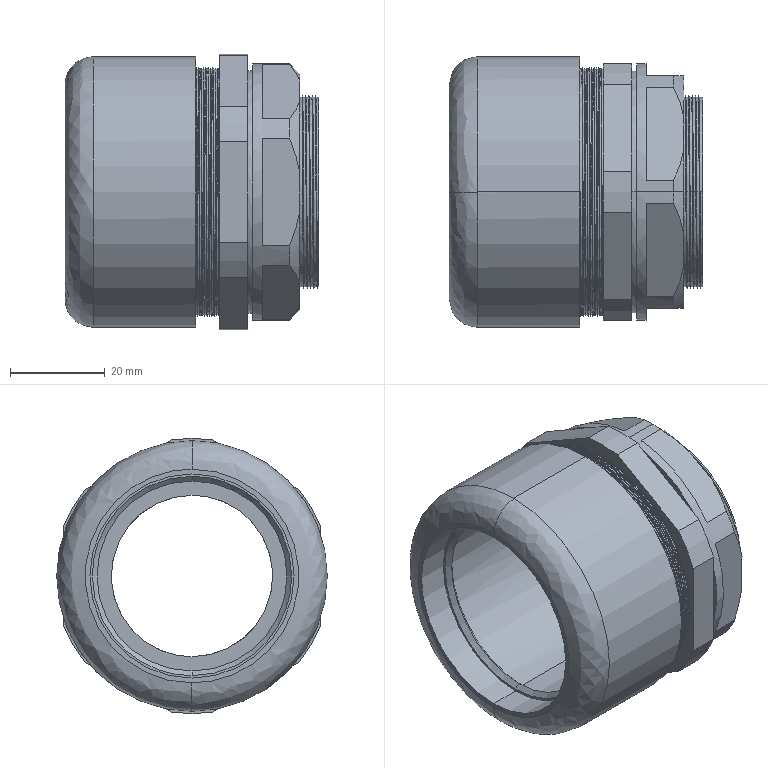Part | SolidWorks | features BaseBody 1 | 1 solid | 106 faces | box 53.5 x 57 x 57.999 mm | volume 57966 mm3 | cylinder 52 | plane 31 | spline 12 | cone 11 | commonest cylinder face diameters 52 x22 40 x11 58 x7 34 x2 42 x2 43 x2